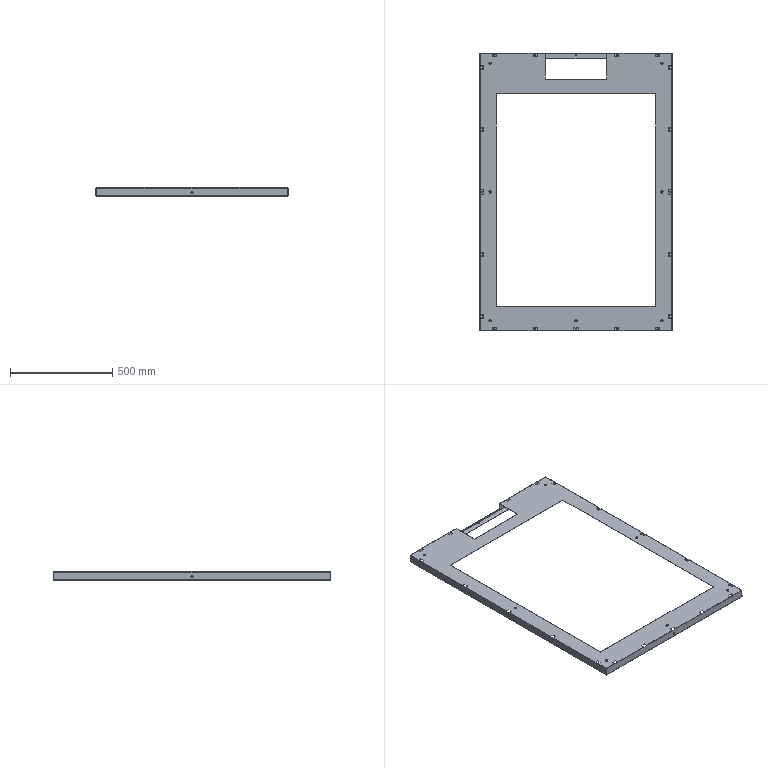Part | SolidWorks | features ICE 8, EdgeFlange 2, FlatPattern 1, SMBaseFlange 1, SheetMetal 1 | 1 solid | 384 faces | box 939 x 1359 x 40 mm | volume 703694 mm3 | plane 242 | cylinder 126 | spline 16 | commonest cylinder face diameters 7 x50 0.4 x28 2.4 x28 11 x14 10 x6